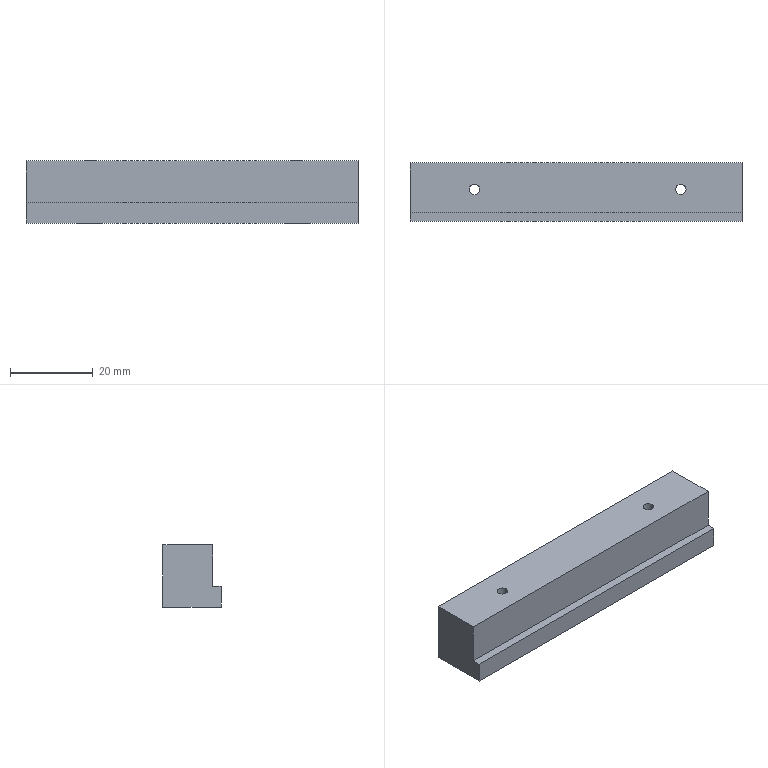Part | STEP file | 1 solid | 24 faces | box 80 x 14 x 15 mm | volume 14919 mm3 | plane 14 | cylinder 10 | commonest cylinder face diameters 6 x6 2.513 x4